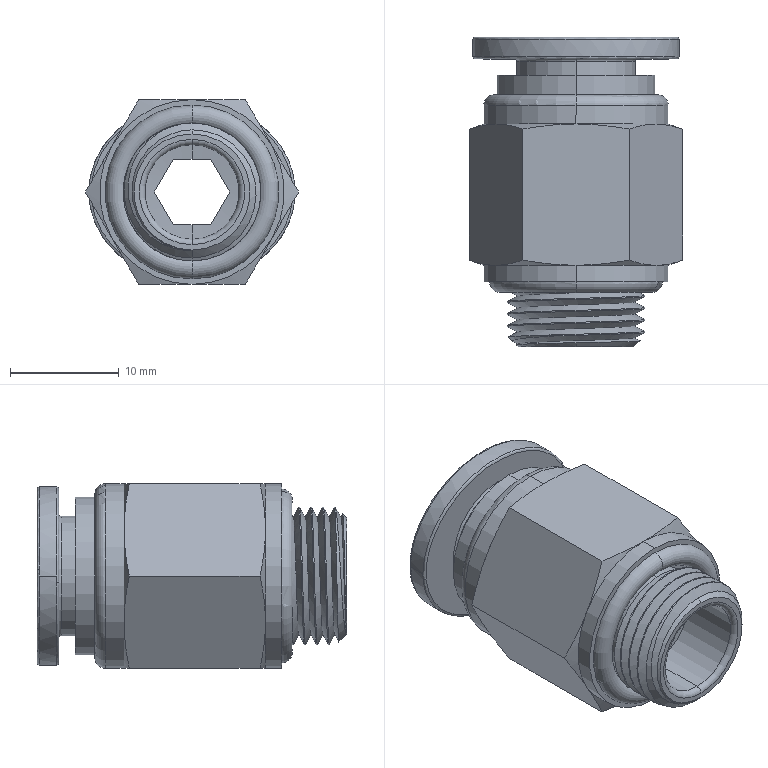Part | STEP file | Quick coupling - 1-4 BSP - COLD | 2 solids | 88 faces | box 19.63 x 28.5 x 17 mm | volume 3780 mm3 | cylinder 27 | cone 21 | plane 20 | torus 12 | spline 8 | commonest cylinder face diameters 12.7 x9 17 x4 8.7 x2 10 x2 10.7 x2 11 x2